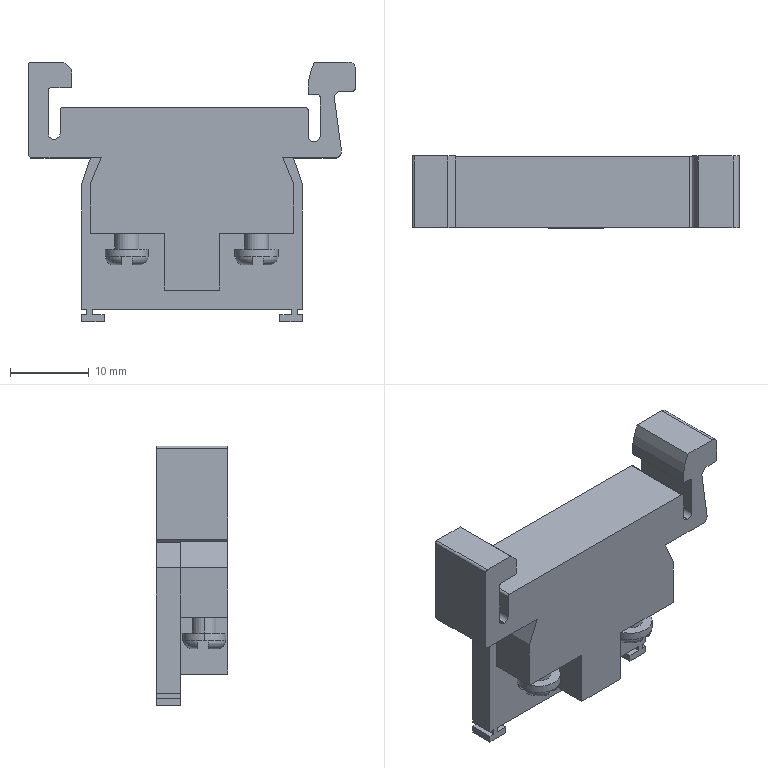Part | STEP file | Short piece 2 | 1 solid | 116 faces | box 41.5 x 9.1 x 33 mm | volume 6155 mm3 | plane 86 | cylinder 21 | torus 8 | other 1 | commonest cylinder face diameters 0.6 x6 1.4 x4 3.085 x4 5.5 x4 0.8 x1 1.6 x1